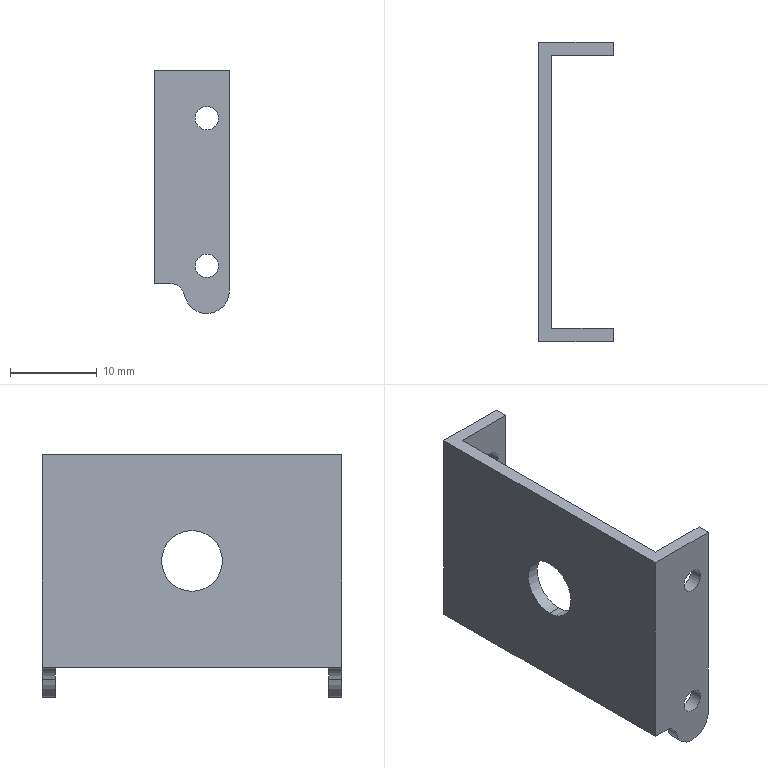Part | SolidWorks | features BaseBody 1 | 1 solid | 24 faces | box 8.6 x 34.5 x 28 mm | volume 1746 mm3 | cylinder 14 | plane 10 | commonest cylinder face diameters 2.7 x8 3.485 x2 5.2 x2 7 x2
STEP:
#1=CARTESIAN_POINT('',(1.5,17.25,-1.757));
#2=VERTEX_POINT('',#1);
#3=CARTESIAN_POINT('',(1.5,17.25,5.243));
#4=VERTEX_POINT('',#3);
#5=CARTESIAN_POINT('',(1.5,17.25,1.743));
#6=DIRECTION('',(-1.,0.,0.));
#7=DIRECTION('',(0.,-1.,0.));
#8=AXIS2_PLACEMENT_3D('',#5,#6,#7);
#9=CIRCLE('',#8,3.5);
#10=EDGE_CURVE('',#2,#4,#9,.T.);
#11=ORIENTED_EDGE('',*,*,#10,.F.);
#12=CARTESIAN_POINT('',(0.,17.25,-1.757));
#13=VERTEX_POINT('',#12);
#14=CARTESIAN_POINT('',(8.6,17.25,-1.757));
#15=DIRECTION('',(-1.,0.,0.));
#16=VECTOR('',#15,1000.);
#17=LINE('',#14,#16);
#18=EDGE_CURVE('',#2,#13,#17,.T.);
#19=ORIENTED_EDGE('',*,*,#18,.T.);
#20=CARTESIAN_POINT('',(0.,17.25,5.243));
#21=VERTEX_POINT('',#20);
#22=CARTESIAN_POINT('',(0.,17.25,1.743));
#23=DIRECTION('',(-1.,0.,0.));
#24=DIRECTION('',(0.,0.,1.));
#25=AXIS2_PLACEMENT_3D('',#22,#23,#24);
#26=CIRCLE('',#25,3.5);
#27=EDGE_CURVE('',#13,#21,#26,.T.);
#28=ORIENTED_EDGE('',*,*,#27,.T.);
#29=CARTESIAN_POINT('',(8.6,17.25,5.243));
#30=DIRECTION('',(-1.,0.,0.));
#31=VECTOR('',#30,1000.);
#32=LINE('',#29,#31);
#33=EDGE_CURVE('',#4,#21,#32,.T.);
#34=ORIENTED_EDGE('',*,*,#33,.F.);
#35=EDGE_LOOP('',(#11,#19,#28,#34));
#36=FACE_OUTER_BOUND('',#35,.T.);
#37=CARTESIAN_POINT('',(8.6,17.25,1.743));
#38=DIRECTION('',(-1.,0.,0.));
#39=DIRECTION('',(0.,0.,1.));
#40=AXIS2_PLACEMENT_3D('',#37,#38,#39);
#41=CYLINDRICAL_SURFACE('',#40,3.5);
#42=ADVANCED_FACE('',(#36),#41,.F.);
#43=CARTESIAN_POINT('',(7.35,0.,8.5));
#44=VERTEX_POINT('',#43);
#45=CARTESIAN_POINT('',(4.65,0.,8.5));
#46=VERTEX_POINT('',#45);
#47=CARTESIAN_POINT('',(6.,0.,8.5));
#48=DIRECTION('',(0.,1.,0.));
#49=DIRECTION('',(-1.,0.,0.));
#50=AXIS2_PLACEMENT_3D('',#47,#48,#49);
#51=CIRCLE('',#50,1.35);
#52=EDGE_CURVE('',#44,#46,#51,.T.);
#53=ORIENTED_EDGE('',*,*,#52,.F.);
#54=CARTESIAN_POINT('',(7.35,1.5,8.5));
#55=VERTEX_POINT('',#54);
#56=CARTESIAN_POINT('',(7.35,0.,8.5));
#57=DIRECTION('',(0.,1.,0.));
#58=VECTOR('',#57,1000.);
#59=LINE('',#56,#58);
#60=EDGE_CURVE('',#44,#55,#59,.T.);
#61=ORIENTED_EDGE('',*,*,#60,.T.);
#62=CARTESIAN_POINT('',(4.65,1.5,8.5));
#63=VERTEX_POINT('',#62);
#64=CARTESIAN_POINT('',(6.,1.5,8.5));
#65=DIRECTION('',(0.,-1.,0.));
#66=DIRECTION('',(0.,0.,-1.));
#67=AXIS2_PLACEMENT_3D('',#64,#65,#66);
#68=CIRCLE('',#67,1.35);
#69=EDGE_CURVE('',#63,#55,#68,.T.);
#70=ORIENTED_EDGE('',*,*,#69,.F.);
#71=CARTESIAN_POINT('',(4.65,0.,8.5));
#72=DIRECTION('',(0.,1.,0.));
#73=VECTOR('',#72,1000.);
#74=LINE('',#71,#73);
#75=EDGE_CURVE('',#46,#63,#74,.T.);
#76=ORIENTED_EDGE('',*,*,#75,.F.);
#77=EDGE_LOOP('',(#53,#61,#70,#76));
#78=FACE_OUTER_BOUND('',#77,.T.);
#79=CARTESIAN_POINT('',(6.,0.,8.5));
#80=DIRECTION('',(0.,1.,0.));
#81=DIRECTION('',(-1.,0.,0.));
#82=AXIS2_PLACEMENT_3D('',#79,#80,#81);
#83=CYLINDRICAL_SURFACE('',#82,1.35);
#84=ADVANCED_FACE('',(#78),#83,.F.);
#85=CARTESIAN_POINT('',(7.35,33.,8.5));
#86=VERTEX_POINT('',#85);
#87=CARTESIAN_POINT('',(4.65,33.,8.5));
#88=VERTEX_POINT('',#87);
#89=CARTESIAN_POINT('',(6.,33.,8.5));
#90=DIRECTION('',(0.,1.,0.));
#91=DIRECTION('',(0.,0.,1.));
#92=AXIS2_PLACEMENT_3D('',#89,#90,#91);
#93=CIRCLE('',#92,1.35);
#94=EDGE_CURVE('',#86,#88,#93,.T.);
#95=ORIENTED_EDGE('',*,*,#94,.F.);
#96=CARTESIAN_POINT('',(7.35,34.5,8.5));
#97=VERTEX_POINT('',#96);
#98=CARTESIAN_POINT('',(7.35,0.,8.5));
#99=DIRECTION('',(0.,1.,0.));
#100=VECTOR('',#99,1000.);
#101=LINE('',#98,#100);
#102=EDGE_CURVE('',#86,#97,#101,.T.);
#103=ORIENTED_EDGE('',*,*,#102,.T.);
#104=CARTESIAN_POINT('',(4.65,34.5,8.5));
#105=VERTEX_POINT('',#104);
#106=CARTESIAN_POINT('',(6.,34.5,8.5));
#107=DIRECTION('',(0.,1.,0.));
#108=DIRECTION('',(-1.,0.,0.));
#109=AXIS2_PLACEMENT_3D('',#106,#107,#108);
#110=CIRCLE('',#109,1.35);
#111=EDGE_CURVE('',#97,#105,#110,.T.);
#112=ORIENTED_EDGE('',*,*,#111,.T.);
#113=CARTESIAN_POINT('',(4.65,0.,8.5));
#114=DIRECTION('',(0.,1.,0.));
#115=VECTOR('',#114,1000.);
#116=LINE('',#113,#115);
#117=EDGE_CURVE('',#88,#105,#116,.T.);
#118=ORIENTED_EDGE('',*,*,#117,.F.);
#119=EDGE_LOOP('',(#95,#103,#112,#118));
#120=FACE_OUTER_BOUND('',#119,.T.);
#121=CARTESIAN_POINT('',(6.,0.,8.5));
#122=DIRECTION('',(0.,1.,0.));
#123=DIRECTION('',(-1.,0.,0.));
#124=AXIS2_PLACEMENT_3D('',#121,#122,#123);
#125=CYLINDRICAL_SURFACE('',#124,1.35);
#126=ADVANCED_FACE('',(#120),#125,.F.);
#127=CARTESIAN_POINT('',(7.35,0.,-8.5));
#128=VERTEX_POINT('',#127);
#129=CARTESIAN_POINT('',(4.65,0.,-8.5));
#130=VERTEX_POINT('',#129);
#131=CARTESIAN_POINT('',(6.,0.,-8.5));
#132=DIRECTION('',(0.,1.,0.));
#133=DIRECTION('',(-1.,0.,0.));
#134=AXIS2_PLACEMENT_3D('',#131,#132,#133);
#135=CIRCLE('',#134,1.35);
#136=EDGE_CURVE('',#128,#130,#135,.T.);
#137=ORIENTED_EDGE('',*,*,#136,.F.);
#138=CARTESIAN_POINT('',(7.35,1.5,-8.5));
#139=VERTEX_POINT('',#138);
#140=CARTESIAN_POINT('',(7.35,0.,-8.5));
#141=DIRECTION('',(0.,1.,0.));
#142=VECTOR('',#141,1000.);
#143=LINE('',#140,#142);
#144=EDGE_CURVE('',#128,#139,#143,.T.);
#145=ORIENTED_EDGE('',*,*,#144,.T.);
#146=CARTESIAN_POINT('',(4.65,1.5,-8.5));
#147=VERTEX_POINT('',#146);
#148=CARTESIAN_POINT('',(6.,1.5,-8.5));
#149=DIRECTION('',(0.,-1.,0.));
#150=DIRECTION('',(0.,0.,-1.));
#151=AXIS2_PLACEMENT_3D('',#148,#149,#150);
#152=CIRCLE('',#151,1.35);
#153=EDGE_CURVE('',#147,#139,#152,.T.);
#154=ORIENTED_EDGE('',*,*,#153,.F.);
#155=CARTESIAN_POINT('',(4.65,0.,-8.5));
#156=DIRECTION('',(0.,1.,0.));
#157=VECTOR('',#156,1000.);
#158=LINE('',#155,#157);
#159=EDGE_CURVE('',#130,#147,#158,.T.);
#160=ORIENTED_EDGE('',*,*,#159,.F.);
#161=EDGE_LOOP('',(#137,#145,#154,#160));
#162=FACE_OUTER_BOUND('',#161,.T.);
#163=CARTESIAN_POINT('',(6.,0.,-8.5));
#164=DIRECTION('',(0.,1.,0.));
#165=DIRECTION('',(-1.,0.,0.));
#166=AXIS2_PLACEMENT_3D('',#163,#164,#165);
#167=CYLINDRICAL_SURFACE('',#166,1.35);
#168=ADVANCED_FACE('',(#162),#167,.F.);
#169=CARTESIAN_POINT('',(7.35,33.,-8.5));
#170=VERTEX_POINT('',#169);
#171=CARTESIAN_POINT('',(4.65,33.,-8.5));
#172=VERTEX_POINT('',#171);
#173=CARTESIAN_POINT('',(6.,33.,-8.5));
#174=DIRECTION('',(0.,1.,0.));
#175=DIRECTION('',(0.,0.,1.));
#176=AXIS2_PLACEMENT_3D('',#173,#174,#175);
#177=CIRCLE('',#176,1.35);
#178=EDGE_CURVE('',#170,#172,#177,.T.);
#179=ORIENTED_EDGE('',*,*,#178,.F.);
#180=CARTESIAN_POINT('',(7.35,34.5,-8.5));
#181=VERTEX_POINT('',#180);
#182=CARTESIAN_POINT('',(7.35,0.,-8.5));
#183=DIRECTION('',(0.,1.,0.));
#184=VECTOR('',#183,1000.);
#185=LINE('',#182,#184);
#186=EDGE_CURVE('',#170,#181,#185,.T.);
#187=ORIENTED_EDGE('',*,*,#186,.T.);
#188=CARTESIAN_POINT('',(4.65,34.5,-8.5));
#189=VERTEX_POINT('',#188);
#190=CARTESIAN_POINT('',(6.,34.5,-8.5));
#191=DIRECTION('',(0.,1.,0.));
#192=DIRECTION('',(-1.,0.,0.));
#193=AXIS2_PLACEMENT_3D('',#190,#191,#192);
#194=CIRCLE('',#193,1.35);
#195=EDGE_CURVE('',#181,#189,#194,.T.);
#196=ORIENTED_EDGE('',*,*,#195,.T.);
#197=CARTESIAN_POINT('',(4.65,0.,-8.5));
#198=DIRECTION('',(0.,1.,0.));
#199=VECTOR('',#198,1000.);
#200=LINE('',#197,#199);
#201=EDGE_CURVE('',#172,#189,#200,.T.);
#202=ORIENTED_EDGE('',*,*,#201,.F.);
#203=EDGE_LOOP('',(#179,#187,#196,#202));
#204=FACE_OUTER_BOUND('',#203,.T.);
#205=CARTESIAN_POINT('',(6.,0.,-8.5));
#206=DIRECTION('',(0.,1.,0.));
#207=DIRECTION('',(-1.,0.,0.));
#208=AXIS2_PLACEMENT_3D('',#205,#206,#207);
#209=CYLINDRICAL_SURFACE('',#208,1.35);
#210=ADVANCED_FACE('',(#204),#209,.F.);
#211=CARTESIAN_POINT('',(6.,0.,8.5));
#212=DIRECTION('',(0.,1.,0.));
#213=DIRECTION('',(-1.,0.,0.));
#214=AXIS2_PLACEMENT_3D('',#211,#212,#213);
#215=CIRCLE('',#214,1.35);
#216=EDGE_CURVE('',#46,#44,#215,.T.);
#217=ORIENTED_EDGE('',*,*,#216,.T.);
#218=ORIENTED_EDGE('',*,*,#52,.T.);
#219=EDGE_LOOP('',(#217,#218));
#220=FACE_BOUND('',#219,.T.);
#221=CARTESIAN_POINT('',(6.,0.,-8.5));
#222=DIRECTION('',(0.,1.,0.));
#223=DIRECTION('',(-1.,0.,0.));
#224=AXIS2_PLACEMENT_3D('',#221,#222,#223);
#225=CIRCLE('',#224,1.35);
#226=EDGE_CURVE('',#130,#128,#225,.T.);
#227=ORIENTED_EDGE('',*,*,#226,.T.);
#228=ORIENTED_EDGE('',*,*,#136,.T.);
#229=EDGE_LOOP('',(#227,#228));
#230=FACE_BOUND('',#229,.T.);
#231=CARTESIAN_POINT('',(8.6,0.,-11.4));
#232=VERTEX_POINT('',#231);
#233=CARTESIAN_POINT('',(3.451,0.,-11.913));
#234=VERTEX_POINT('',#233);
#235=CARTESIAN_POINT('',(6.,0.,-11.4));
#236=DIRECTION('',(0.,1.,0.));
#237=DIRECTION('',(0.,0.,1.));
#238=AXIS2_PLACEMENT_3D('',#235,#236,#237);
#239=CIRCLE('',#238,2.6);
#240=EDGE_CURVE('',#232,#234,#239,.T.);
#241=ORIENTED_EDGE('',*,*,#240,.F.);
#242=CARTESIAN_POINT('',(8.6,0.,14.));
#243=VERTEX_POINT('',#242);
#244=CARTESIAN_POINT('',(8.6,0.,14.));
#245=DIRECTION('',(0.,0.,-1.));
#246=VECTOR('',#245,1000.);
#247=LINE('',#244,#246);
#248=EDGE_CURVE('',#243,#232,#247,.T.);
#249=ORIENTED_EDGE('',*,*,#248,.F.);
#250=CARTESIAN_POINT('',(0.,0.,14.));
#251=VERTEX_POINT('',#250);
#252=CARTESIAN_POINT('',(8.6,0.,14.));
#253=DIRECTION('',(1.,0.,0.));
#254=VECTOR('',#253,1000.);
#255=LINE('',#252,#254);
#256=EDGE_CURVE('',#251,#243,#255,.T.);
#257=ORIENTED_EDGE('',*,*,#256,.F.);
#258=CARTESIAN_POINT('',(0.,0.,-10.515));
#259=VERTEX_POINT('',#258);
#260=CARTESIAN_POINT('',(0.,0.,14.));
#261=DIRECTION('',(0.,0.,-1.));
#262=VECTOR('',#261,1000.);
#263=LINE('',#260,#262);
#264=EDGE_CURVE('',#251,#259,#263,.T.);
#265=ORIENTED_EDGE('',*,*,#264,.T.);
#266=CARTESIAN_POINT('',(1.743,0.,-10.515));
#267=VERTEX_POINT('',#266);
#268=CARTESIAN_POINT('',(0.,0.,-10.515));
#269=DIRECTION('',(-1.,0.,0.));
#270=VECTOR('',#269,1000.);
#271=LINE('',#268,#270);
#272=EDGE_CURVE('',#267,#259,#271,.T.);
#273=ORIENTED_EDGE('',*,*,#272,.F.);
#274=CARTESIAN_POINT('',(1.743,0.,-12.257));
#275=DIRECTION('',(0.,1.,0.));
#276=DIRECTION('',(0.,0.,1.));
#277=AXIS2_PLACEMENT_3D('',#274,#275,#276);
#278=CIRCLE('',#277,1.743);
#279=EDGE_CURVE('',#267,#234,#278,.T.);
#280=ORIENTED_EDGE('',*,*,#279,.T.);
#281=EDGE_LOOP('',(#241,#249,#257,#265,#273,#280));
#282=FACE_OUTER_BOUND('',#281,.T.);
#283=CARTESIAN_POINT('',(8.6,0.,14.));
#284=DIRECTION('',(0.,1.,0.));
#285=DIRECTION('',(-1.,0.,0.));
#286=AXIS2_PLACEMENT_3D('',#283,#284,#285);
#287=PLANE('',#286);
#288=ADVANCED_FACE('',(#220,#230,#282),#287,.F.);
#289=ORIENTED_EDGE('',*,*,#69,.T.);
#290=CARTESIAN_POINT('',(6.,1.5,8.5));
#291=DIRECTION('',(0.,-1.,0.));
#292=DIRECTION('',(0.,0.,-1.));
#293=AXIS2_PLACEMENT_3D('',#290,#291,#292);
#294=CIRCLE('',#293,1.35);
#295=EDGE_CURVE('',#55,#63,#294,.T.);
#296=ORIENTED_EDGE('',*,*,#295,.T.);
#297=EDGE_LOOP('',(#289,#296));
#298=FACE_BOUND('',#297,.T.);
#299=ORIENTED_EDGE('',*,*,#153,.T.);
#300=CARTESIAN_POINT('',(6.,1.5,-8.5));
#301=DIRECTION('',(0.,-1.,0.));
#302=DIRECTION('',(0.,0.,-1.));
#303=AXIS2_PLACEMENT_3D('',#300,#301,#302);
#304=CIRCLE('',#303,1.35);
#305=EDGE_CURVE('',#139,#147,#304,.T.);
#306=ORIENTED_EDGE('',*,*,#305,.T.);
#307=EDGE_LOOP('',(#299,#306));
#308=FACE_BOUND('',#307,.T.);
#309=CARTESIAN_POINT('',(8.6,1.5,14.));
#310=VERTEX_POINT('',#309);
#311=CARTESIAN_POINT('',(8.6,1.5,-11.4));
#312=VERTEX_POINT('',#311);
#313=CARTESIAN_POINT('',(8.6,1.5,14.));
#314=DIRECTION('',(0.,0.,-1.));
#315=VECTOR('',#314,1000.);
#316=LINE('',#313,#315);
#317=EDGE_CURVE('',#310,#312,#316,.T.);
#318=ORIENTED_EDGE('',*,*,#317,.T.);
#319=CARTESIAN_POINT('',(3.451,1.5,-11.913));
#320=VERTEX_POINT('',#319);
#321=CARTESIAN_POINT('',(6.,1.5,-11.4));
#322=DIRECTION('',(0.,-1.,0.));
#323=DIRECTION('',(0.,0.,-1.));
#324=AXIS2_PLACEMENT_3D('',#321,#322,#323);
#325=CIRCLE('',#324,2.6);
#326=EDGE_CURVE('',#320,#312,#325,.T.);
#327=ORIENTED_EDGE('',*,*,#326,.F.);
#328=CARTESIAN_POINT('',(1.743,1.5,-10.515));
#329=VERTEX_POINT('',#328);
#330=CARTESIAN_POINT('',(1.743,1.5,-12.257));
#331=DIRECTION('',(0.,-1.,0.));
#332=DIRECTION('',(0.,0.,-1.));
#333=AXIS2_PLACEMENT_3D('',#330,#331,#332);
#334=CIRCLE('',#333,1.743);
#335=EDGE_CURVE('',#320,#329,#334,.T.);
#336=ORIENTED_EDGE('',*,*,#335,.T.);
#337=CARTESIAN_POINT('',(1.5,1.5,-10.515));
#338=VERTEX_POINT('',#337);
#339=CARTESIAN_POINT('',(1.5,1.5,-10.515));
#340=DIRECTION('',(1.,0.,0.));
#341=VECTOR('',#340,1000.);
#342=LINE('',#339,#341);
#343=EDGE_CURVE('',#338,#329,#342,.T.);
#344=ORIENTED_EDGE('',*,*,#343,.F.);
#345=CARTESIAN_POINT('',(1.5,1.5,14.));
#346=VERTEX_POINT('',#345);
#347=CARTESIAN_POINT('',(1.5,1.5,14.));
#348=DIRECTION('',(0.,0.,-1.));
#349=VECTOR('',#348,1000.);
#350=LINE('',#347,#349);
#351=EDGE_CURVE('',#346,#338,#350,.T.);
#352=ORIENTED_EDGE('',*,*,#351,.F.);
#353=CARTESIAN_POINT('',(1.5,1.5,14.));
#354=DIRECTION('',(-1.,0.,0.));
#355=VECTOR('',#354,1000.);
#356=LINE('',#353,#355);
#357=EDGE_CURVE('',#310,#346,#356,.T.);
#358=ORIENTED_EDGE('',*,*,#357,.F.);
#359=EDGE_LOOP('',(#318,#327,#336,#344,#352,#358));
#360=FACE_OUTER_BOUND('',#359,.T.);
#361=CARTESIAN_POINT('',(1.5,1.5,14.));
#362=DIRECTION('',(0.,-1.,0.));
#363=DIRECTION('',(0.,0.,-1.));
#364=AXIS2_PLACEMENT_3D('',#361,#362,#363);
#365=PLANE('',#364);
#366=ADVANCED_FACE('',(#298,#308,#360),#365,.F.);
#367=CARTESIAN_POINT('',(1.5,17.25,1.743));
#368=DIRECTION('',(-1.,0.,0.));
#369=DIRECTION('',(0.,-1.,0.));
#370=AXIS2_PLACEMENT_3D('',#367,#368,#369);
#371=CIRCLE('',#370,3.5);
#372=EDGE_CURVE('',#4,#2,#371,.T.);
#373=ORIENTED_EDGE('',*,*,#372,.T.);
#374=ORIENTED_EDGE('',*,*,#10,.T.);
#375=EDGE_LOOP('',(#373,#374));
#376=FACE_BOUND('',#375,.T.);
#377=CARTESIAN_POINT('',(1.5,33.,-10.515));
#378=VERTEX_POINT('',#377);
#379=CARTESIAN_POINT('',(1.5,33.,-10.515));
#380=DIRECTION('',(0.,-1.,0.));
#381=VECTOR('',#380,1000.);
#382=LINE('',#379,#381);
#383=EDGE_CURVE('',#378,#338,#382,.T.);
#384=ORIENTED_EDGE('',*,*,#383,.F.);
#385=CARTESIAN_POINT('',(1.5,33.,14.));
#386=VERTEX_POINT('',#385);
#387=CARTESIAN_POINT('',(1.5,33.,14.));
#388=DIRECTION('',(0.,0.,-1.));
#389=VECTOR('',#388,1000.);
#390=LINE('',#387,#389);
#391=EDGE_CURVE('',#386,#378,#390,.T.);
#392=ORIENTED_EDGE('',*,*,#391,.F.);
#393=CARTESIAN_POINT('',(1.5,33.,14.));
#394=DIRECTION('',(0.,1.,0.));
#395=VECTOR('',#394,1000.);
#396=LINE('',#393,#395);
#397=EDGE_CURVE('',#346,#386,#396,.T.);
#398=ORIENTED_EDGE('',*,*,#397,.F.);
#399=ORIENTED_EDGE('',*,*,#351,.T.);
#400=EDGE_LOOP('',(#384,#392,#398,#399));
#401=FACE_OUTER_BOUND('',#400,.T.);
#402=CARTESIAN_POINT('',(1.5,33.,14.));
#403=DIRECTION('',(-1.,0.,0.));
#404=DIRECTION('',(0.,-1.,0.));
#405=AXIS2_PLACEMENT_3D('',#402,#403,#404);
#406=PLANE('',#405);
#407=ADVANCED_FACE('',(#376,#401),#406,.F.);
#408=CARTESIAN_POINT('',(6.,33.,8.5));
#409=DIRECTION('',(0.,1.,0.));
#410=DIRECTION('',(0.,0.,1.));
#411=AXIS2_PLACEMENT_3D('',#408,#409,#410);
#412=CIRCLE('',#411,1.35);
#413=EDGE_CURVE('',#88,#86,#412,.T.);
#414=ORIENTED_EDGE('',*,*,#413,.T.);
#415=ORIENTED_EDGE('',*,*,#94,.T.);
#416=EDGE_LOOP('',(#414,#415));
#417=FACE_BOUND('',#416,.T.);
#418=CARTESIAN_POINT('',(6.,33.,-8.5));
#419=DIRECTION('',(0.,1.,0.));
#420=DIRECTION('',(0.,0.,1.));
#421=AXIS2_PLACEMENT_3D('',#418,#419,#420);
#422=CIRCLE('',#421,1.35);
#423=EDGE_CURVE('',#172,#170,#422,.T.);
#424=ORIENTED_EDGE('',*,*,#423,.T.);
#425=ORIENTED_EDGE('',*,*,#178,.T.);
#426=EDGE_LOOP('',(#424,#425));
#427=FACE_BOUND('',#426,.T.);
#428=CARTESIAN_POINT('',(8.6,33.,-11.4));
#429=VERTEX_POINT('',#428);
#430=CARTESIAN_POINT('',(3.451,33.,-11.913));
#431=VERTEX_POINT('',#430);
#432=CARTESIAN_POINT('',(6.,33.,-11.4));
#433=DIRECTION('',(0.,1.,0.));
#434=DIRECTION('',(0.,0.,1.));
#435=AXIS2_PLACEMENT_3D('',#432,#433,#434);
#436=CIRCLE('',#435,2.6);
#437=EDGE_CURVE('',#429,#431,#436,.T.);
#438=ORIENTED_EDGE('',*,*,#437,.F.);
#439=CARTESIAN_POINT('',(8.6,33.,14.));
#440=VERTEX_POINT('',#439);
#441=CARTESIAN_POINT('',(8.6,33.,14.));
#442=DIRECTION('',(0.,0.,-1.));
#443=VECTOR('',#442,1000.);
#444=LINE('',#441,#443);
#445=EDGE_CURVE('',#440,#429,#444,.T.);
#446=ORIENTED_EDGE('',*,*,#445,.F.);
#447=CARTESIAN_POINT('',(8.6,33.,14.));
#448=DIRECTION('',(1.,0.,0.));
#449=VECTOR('',#448,1000.);
#450=LINE('',#447,#449);
#451=EDGE_CURVE('',#386,#440,#450,.T.);
#452=ORIENTED_EDGE('',*,*,#451,.F.);
#453=ORIENTED_EDGE('',*,*,#391,.T.);
#454=CARTESIAN_POINT('',(1.743,33.,-10.515));
#455=VERTEX_POINT('',#454);
#456=CARTESIAN_POINT('',(8.6,33.,-10.515));
#457=DIRECTION('',(-1.,0.,0.));
#458=VECTOR('',#457,1000.);
#459=LINE('',#456,#458);
#460=EDGE_CURVE('',#455,#378,#459,.T.);
#461=ORIENTED_EDGE('',*,*,#460,.F.);
#462=CARTESIAN_POINT('',(1.743,33.,-12.257));
#463=DIRECTION('',(0.,1.,0.));
#464=DIRECTION('',(0.,0.,1.));
#465=AXIS2_PLACEMENT_3D('',#462,#463,#464);
#466=CIRCLE('',#465,1.743);
#467=EDGE_CURVE('',#455,#431,#466,.T.);
#468=ORIENTED_EDGE('',*,*,#467,.T.);
#469=EDGE_LOOP('',(#438,#446,#452,#453,#461,#468));
#470=FACE_OUTER_BOUND('',#469,.T.);
#471=CARTESIAN_POINT('',(8.6,33.,14.));
#472=DIRECTION('',(0.,1.,0.));
#473=DIRECTION('',(0.,0.,1.));
#474=AXIS2_PLACEMENT_3D('',#471,#472,#473);
#475=PLANE('',#474);
#476=ADVANCED_FACE('',(#417,#427,#470),#475,.F.);
#477=CARTESIAN_POINT('',(6.,34.5,8.5));
#478=DIRECTION('',(0.,1.,0.));
#479=DIRECTION('',(-1.,0.,0.));
#480=AXIS2_PLACEMENT_3D('',#477,#478,#479);
#481=CIRCLE('',#480,1.35);
#482=EDGE_CURVE('',#105,#97,#481,.T.);
#483=ORIENTED_EDGE('',*,*,#482,.F.);
#484=ORIENTED_EDGE('',*,*,#111,.F.);
#485=EDGE_LOOP('',(#483,#484));
#486=FACE_BOUND('',#485,.T.);
#487=CARTESIAN_POINT('',(6.,34.5,-8.5));
#488=DIRECTION('',(0.,1.,0.));
#489=DIRECTION('',(-1.,0.,0.));
#490=AXIS2_PLACEMENT_3D('',#487,#488,#489);
#491=CIRCLE('',#490,1.35);
#492=EDGE_CURVE('',#189,#181,#491,.T.);
#493=ORIENTED_EDGE('',*,*,#492,.F.);
#494=ORIENTED_EDGE('',*,*,#195,.F.);
#495=EDGE_LOOP('',(#493,#494));
#496=FACE_BOUND('',#495,.T.);
#497=CARTESIAN_POINT('',(8.6,34.5,-11.4));
#498=VERTEX_POINT('',#497);
#499=CARTESIAN_POINT('',(3.451,34.5,-11.913));
#500=VERTEX_POINT('',#499);
#501=CARTESIAN_POINT('',(6.,34.5,-11.4));
#502=DIRECTION('',(0.,1.,0.));
#503=DIRECTION('',(0.,0.,1.));
#504=AXIS2_PLACEMENT_3D('',#501,#502,#503);
#505=CIRCLE('',#504,2.6);
#506=EDGE_CURVE('',#498,#500,#505,.T.);
#507=ORIENTED_EDGE('',*,*,#506,.T.);
#508=CARTESIAN_POINT('',(1.743,34.5,-10.515));
#509=VERTEX_POINT('',#508);
#510=CARTESIAN_POINT('',(1.743,34.5,-12.257));
#511=DIRECTION('',(0.,1.,0.));
#512=DIRECTION('',(0.,0.,1.));
#513=AXIS2_PLACEMENT_3D('',#510,#511,#512);
#514=CIRCLE('',#513,1.743);
#515=EDGE_CURVE('',#509,#500,#514,.T.);
#516=ORIENTED_EDGE('',*,*,#515,.F.);
#517=CARTESIAN_POINT('',(0.,34.5,-10.515));
#518=VERTEX_POINT('',#517);
#519=CARTESIAN_POINT('',(0.,34.5,-10.515));
#520=DIRECTION('',(-1.,0.,0.));
#521=VECTOR('',#520,1000.);
#522=LINE('',#519,#521);
#523=EDGE_CURVE('',#509,#518,#522,.T.);
#524=ORIENTED_EDGE('',*,*,#523,.T.);
#525=CARTESIAN_POINT('',(0.,34.5,14.));
#526=VERTEX_POINT('',#525);
#527=CARTESIAN_POINT('',(0.,34.5,14.));
#528=DIRECTION('',(0.,0.,-1.));
#529=VECTOR('',#528,1000.);
#530=LINE('',#527,#529);
#531=EDGE_CURVE('',#526,#518,#530,.T.);
#532=ORIENTED_EDGE('',*,*,#531,.F.);
#533=CARTESIAN_POINT('',(8.6,34.5,14.));
#534=VERTEX_POINT('',#533);
#535=CARTESIAN_POINT('',(0.,34.5,14.));
#536=DIRECTION('',(-1.,0.,0.));
#537=VECTOR('',#536,1000.);
#538=LINE('',#535,#537);
#539=EDGE_CURVE('',#534,#526,#538,.T.);
#540=ORIENTED_EDGE('',*,*,#539,.F.);
#541=CARTESIAN_POINT('',(8.6,34.5,14.));
#542=DIRECTION('',(0.,0.,-1.));
#543=VECTOR('',#542,1000.);
#544=LINE('',#541,#543);
#545=EDGE_CURVE('',#534,#498,#544,.T.);
#546=ORIENTED_EDGE('',*,*,#545,.T.);
#547=EDGE_LOOP('',(#507,#516,#524,#532,#540,#546));
#548=FACE_OUTER_BOUND('',#547,.T.);
#549=CARTESIAN_POINT('',(0.,34.5,14.));
#550=DIRECTION('',(0.,-1.,0.));
#551=DIRECTION('',(0.,0.,-1.));
#552=AXIS2_PLACEMENT_3D('',#549,#550,#551);
#553=PLANE('',#552);
#554=ADVANCED_FACE('',(#486,#496,#548),#553,.F.);
#555=CARTESIAN_POINT('',(0.,17.25,1.743));
#556=DIRECTION('',(-1.,0.,0.));
#557=DIRECTION('',(0.,0.,1.));
#558=AXIS2_PLACEMENT_3D('',#555,#556,#557);
#559=CIRCLE('',#558,3.5);
#560=EDGE_CURVE('',#21,#13,#559,.T.);
#561=ORIENTED_EDGE('',*,*,#560,.F.);
#562=ORIENTED_EDGE('',*,*,#27,.F.);
#563=EDGE_LOOP('',(#561,#562));
#564=FACE_BOUND('',#563,.T.);
#565=CARTESIAN_POINT('',(0.,0.,-10.515));
#566=DIRECTION('',(0.,1.,0.));
#567=VECTOR('',#566,1000.);
#568=LINE('',#565,#567);
#569=EDGE_CURVE('',#259,#518,#568,.T.);
#570=ORIENTED_EDGE('',*,*,#569,.F.);
#571=ORIENTED_EDGE('',*,*,#264,.F.);
#572=CARTESIAN_POINT('',(0.,0.,14.));
#573=DIRECTION('',(0.,-1.,0.));
#574=VECTOR('',#573,1000.);
#575=LINE('',#572,#574);
#576=EDGE_CURVE('',#526,#251,#575,.T.);
#577=ORIENTED_EDGE('',*,*,#576,.F.);
#578=ORIENTED_EDGE('',*,*,#531,.T.);
#579=EDGE_LOOP('',(#570,#571,#577,#578));
#580=FACE_OUTER_BOUND('',#579,.T.);
#581=CARTESIAN_POINT('',(0.,0.,14.));
#582=DIRECTION('',(1.,0.,0.));
#583=DIRECTION('',(0.,0.,-1.));
#584=AXIS2_PLACEMENT_3D('',#581,#582,#583);
#585=PLANE('',#584);
#586=ADVANCED_FACE('',(#564,#580),#585,.F.);
#587=ORIENTED_EDGE('',*,*,#248,.T.);
#588=CARTESIAN_POINT('',(8.6,0.,-11.4));
#589=DIRECTION('',(0.,1.,0.));
#590=VECTOR('',#589,1000.);
#591=LINE('',#588,#590);
#592=EDGE_CURVE('',#232,#312,#591,.T.);
#593=ORIENTED_EDGE('',*,*,#592,.T.);
#594=ORIENTED_EDGE('',*,*,#317,.F.);
#595=CARTESIAN_POINT('',(8.6,1.5,14.));
#596=DIRECTION('',(0.,1.,0.));
#597=VECTOR('',#596,1000.);
#598=LINE('',#595,#597);
#599=EDGE_CURVE('',#243,#310,#598,.T.);
#600=ORIENTED_EDGE('',*,*,#599,.F.);
#601=EDGE_LOOP('',(#587,#593,#594,#600));
#602=FACE_OUTER_BOUND('',#601,.T.);
#603=CARTESIAN_POINT('',(8.6,1.5,14.));
#604=DIRECTION('',(-1.,0.,0.));
#605=DIRECTION('',(0.,0.,1.));
#606=AXIS2_PLACEMENT_3D('',#603,#604,#605);
#607=PLANE('',#606);
#608=ADVANCED_FACE('',(#602),#607,.F.);
#609=ORIENTED_EDGE('',*,*,#445,.T.);
#610=CARTESIAN_POINT('',(8.6,0.,-11.4));
#611=DIRECTION('',(0.,1.,0.));
#612=VECTOR('',#611,1000.);
#613=LINE('',#610,#612);
#614=EDGE_CURVE('',#429,#498,#613,.T.);
#615=ORIENTED_EDGE('',*,*,#614,.T.);
#616=ORIENTED_EDGE('',*,*,#545,.F.);
#617=CARTESIAN_POINT('',(8.6,34.5,14.));
#618=DIRECTION('',(0.,1.,0.));
#619=VECTOR('',#618,1000.);
#620=LINE('',#617,#619);
#621=EDGE_CURVE('',#440,#534,#620,.T.);
#622=ORIENTED_EDGE('',*,*,#621,.F.);
#623=EDGE_LOOP('',(#609,#615,#616,#622));
#624=FACE_OUTER_BOUND('',#623,.T.);
#625=CARTESIAN_POINT('',(8.6,34.5,14.));
#626=DIRECTION('',(-1.,0.,0.));
#627=DIRECTION('',(0.,-1.,0.));
#628=AXIS2_PLACEMENT_3D('',#625,#626,#627);
#629=PLANE('',#628);
#630=ADVANCED_FACE('',(#624),#629,.F.);
#631=ORIENTED_EDGE('',*,*,#256,.T.);
#632=ORIENTED_EDGE('',*,*,#599,.T.);
#633=ORIENTED_EDGE('',*,*,#357,.T.);
#634=ORIENTED_EDGE('',*,*,#397,.T.);
#635=ORIENTED_EDGE('',*,*,#451,.T.);
#636=ORIENTED_EDGE('',*,*,#621,.T.);
#637=ORIENTED_EDGE('',*,*,#539,.T.);
#638=ORIENTED_EDGE('',*,*,#576,.T.);
#639=EDGE_LOOP('',(#631,#632,#633,#634,#635,#636,#637,#638));
#640=FACE_OUTER_BOUND('',#639,.T.);
#641=CARTESIAN_POINT('',(0.,0.,14.));
#642=DIRECTION('',(0.,0.,-1.));
#643=DIRECTION('',(-1.,0.,0.));
#644=AXIS2_PLACEMENT_3D('',#641,#642,#643);
#645=PLANE('',#644);
#646=ADVANCED_FACE('',(#640),#645,.F.);
#647=ORIENTED_EDGE('',*,*,#186,.F.);
#648=ORIENTED_EDGE('',*,*,#423,.F.);
#649=ORIENTED_EDGE('',*,*,#201,.T.);
#650=ORIENTED_EDGE('',*,*,#492,.T.);
#651=EDGE_LOOP('',(#647,#648,#649,#650));
#652=FACE_OUTER_BOUND('',#651,.T.);
#653=CARTESIAN_POINT('',(6.,0.,-8.5));
#654=DIRECTION('',(0.,1.,0.));
#655=DIRECTION('',(-1.,0.,0.));
#656=AXIS2_PLACEMENT_3D('',#653,#654,#655);
#657=CYLINDRICAL_SURFACE('',#656,1.35);
#658=ADVANCED_FACE('',(#652),#657,.F.);
#659=ORIENTED_EDGE('',*,*,#144,.F.);
#660=ORIENTED_EDGE('',*,*,#226,.F.);
#661=ORIENTED_EDGE('',*,*,#159,.T.);
#662=ORIENTED_EDGE('',*,*,#305,.F.);
#663=EDGE_LOOP('',(#659,#660,#661,#662));
#664=FACE_OUTER_BOUND('',#663,.T.);
#665=CARTESIAN_POINT('',(6.,0.,-8.5));
#666=DIRECTION('',(0.,1.,0.));
#667=DIRECTION('',(-1.,0.,0.));
#668=AXIS2_PLACEMENT_3D('',#665,#666,#667);
#669=CYLINDRICAL_SURFACE('',#668,1.35);
#670=ADVANCED_FACE('',(#664),#669,.F.);
#671=ORIENTED_EDGE('',*,*,#102,.F.);
#672=ORIENTED_EDGE('',*,*,#413,.F.);
#673=ORIENTED_EDGE('',*,*,#117,.T.);
#674=ORIENTED_EDGE('',*,*,#482,.T.);
#675=EDGE_LOOP('',(#671,#672,#673,#674));
#676=FACE_OUTER_BOUND('',#675,.T.);
#677=CARTESIAN_POINT('',(6.,0.,8.5));
#678=DIRECTION('',(0.,1.,0.));
#679=DIRECTION('',(-1.,0.,0.));
#680=AXIS2_PLACEMENT_3D('',#677,#678,#679);
#681=CYLINDRICAL_SURFACE('',#680,1.35);
#682=ADVANCED_FACE('',(#676),#681,.F.);
#683=ORIENTED_EDGE('',*,*,#60,.F.);
#684=ORIENTED_EDGE('',*,*,#216,.F.);
#685=ORIENTED_EDGE('',*,*,#75,.T.);
#686=ORIENTED_EDGE('',*,*,#295,.F.);
#687=EDGE_LOOP('',(#683,#684,#685,#686));
#688=FACE_OUTER_BOUND('',#687,.T.);
#689=CARTESIAN_POINT('',(6.,0.,8.5));
#690=DIRECTION('',(0.,1.,0.));
#691=DIRECTION('',(-1.,0.,0.));
#692=AXIS2_PLACEMENT_3D('',#689,#690,#691);
#693=CYLINDRICAL_SURFACE('',#692,1.35);
#694=ADVANCED_FACE('',(#688),#693,.F.);
#695=CARTESIAN_POINT('',(3.451,0.,-11.913));
#696=DIRECTION('',(0.,1.,0.));
#697=VECTOR('',#696,1000.);
#698=LINE('',#695,#697);
#699=EDGE_CURVE('',#234,#320,#698,.T.);
#700=ORIENTED_EDGE('',*,*,#699,.F.);
#701=ORIENTED_EDGE('',*,*,#279,.F.);
#702=CARTESIAN_POINT('',(1.743,0.,-10.515));
#703=DIRECTION('',(0.,1.,0.));
#704=VECTOR('',#703,1000.);
#705=LINE('',#702,#704);
#706=EDGE_CURVE('',#267,#329,#705,.T.);
#707=ORIENTED_EDGE('',*,*,#706,.T.);
#708=ORIENTED_EDGE('',*,*,#335,.F.);
#709=EDGE_LOOP('',(#700,#701,#707,#708));
#710=FACE_OUTER_BOUND('',#709,.T.);
#711=CARTESIAN_POINT('',(1.743,0.,-12.257));
#712=DIRECTION('',(0.,1.,0.));
#713=DIRECTION('',(0.,0.,1.));
#714=AXIS2_PLACEMENT_3D('',#711,#712,#713);
#715=CYLINDRICAL_SURFACE('',#714,1.743);
#716=ADVANCED_FACE('',(#710),#715,.F.);
#717=CARTESIAN_POINT('',(1.743,0.,-10.515));
#718=DIRECTION('',(0.,1.,0.));
#719=VECTOR('',#718,1000.);
#720=LINE('',#717,#719);
#721=EDGE_CURVE('',#455,#509,#720,.T.);
#722=ORIENTED_EDGE('',*,*,#721,.T.);
#723=ORIENTED_EDGE('',*,*,#515,.T.);
#724=CARTESIAN_POINT('',(3.451,0.,-11.913));
#725=DIRECTION('',(0.,1.,0.));
#726=VECTOR('',#725,1000.);
#727=LINE('',#724,#726);
#728=EDGE_CURVE('',#431,#500,#727,.T.);
#729=ORIENTED_EDGE('',*,*,#728,.F.);
#730=ORIENTED_EDGE('',*,*,#467,.F.);
#731=EDGE_LOOP('',(#722,#723,#729,#730));
#732=FACE_OUTER_BOUND('',#731,.T.);
#733=CARTESIAN_POINT('',(1.743,0.,-12.257));
#734=DIRECTION('',(0.,1.,0.));
#735=DIRECTION('',(0.,0.,1.));
#736=AXIS2_PLACEMENT_3D('',#733,#734,#735);
#737=CYLINDRICAL_SURFACE('',#736,1.743);
#738=ADVANCED_FACE('',(#732),#737,.F.);
#739=ORIENTED_EDGE('',*,*,#343,.T.);
#740=ORIENTED_EDGE('',*,*,#706,.F.);
#741=ORIENTED_EDGE('',*,*,#272,.T.);
#742=ORIENTED_EDGE('',*,*,#569,.T.);
#743=ORIENTED_EDGE('',*,*,#523,.F.);
#744=ORIENTED_EDGE('',*,*,#721,.F.);
#745=ORIENTED_EDGE('',*,*,#460,.T.);
#746=ORIENTED_EDGE('',*,*,#383,.T.);
#747=EDGE_LOOP('',(#739,#740,#741,#742,#743,#744,#745,#746));
#748=FACE_OUTER_BOUND('',#747,.T.);
#749=CARTESIAN_POINT('',(0.,0.,-10.515));
#750=DIRECTION('',(0.,0.,-1.));
#751=DIRECTION('',(-1.,0.,0.));
#752=AXIS2_PLACEMENT_3D('',#749,#750,#751);
#753=PLANE('',#752);
#754=ADVANCED_FACE('',(#748),#753,.T.);
#755=ORIENTED_EDGE('',*,*,#326,.T.);
#756=ORIENTED_EDGE('',*,*,#592,.F.);
#757=ORIENTED_EDGE('',*,*,#240,.T.);
#758=ORIENTED_EDGE('',*,*,#699,.T.);
#759=EDGE_LOOP('',(#755,#756,#757,#758));
#760=FACE_OUTER_BOUND('',#759,.T.);
#761=CARTESIAN_POINT('',(6.,0.,-11.4));
#762=DIRECTION('',(0.,1.,0.));
#763=DIRECTION('',(0.,0.,1.));
#764=AXIS2_PLACEMENT_3D('',#761,#762,#763);
#765=CYLINDRICAL_SURFACE('',#764,2.6);
#766=ADVANCED_FACE('',(#760),#765,.T.);
#767=ORIENTED_EDGE('',*,*,#437,.T.);
#768=ORIENTED_EDGE('',*,*,#728,.T.);
#769=ORIENTED_EDGE('',*,*,#506,.F.);
#770=ORIENTED_EDGE('',*,*,#614,.F.);
#771=EDGE_LOOP('',(#767,#768,#769,#770));
#772=FACE_OUTER_BOUND('',#771,.T.);
#773=CARTESIAN_POINT('',(6.,0.,-11.4));
#774=DIRECTION('',(0.,1.,0.));
#775=DIRECTION('',(0.,0.,1.));
#776=AXIS2_PLACEMENT_3D('',#773,#774,#775);
#777=CYLINDRICAL_SURFACE('',#776,2.6);
#778=ADVANCED_FACE('',(#772),#777,.T.);
#779=ORIENTED_EDGE('',*,*,#18,.F.);
#780=ORIENTED_EDGE('',*,*,#372,.F.);
#781=ORIENTED_EDGE('',*,*,#33,.T.);
#782=ORIENTED_EDGE('',*,*,#560,.T.);
#783=EDGE_LOOP('',(#779,#780,#781,#782));
#784=FACE_OUTER_BOUND('',#783,.T.);
#785=CARTESIAN_POINT('',(8.6,17.25,1.743));
#786=DIRECTION('',(-1.,0.,0.));
#787=DIRECTION('',(0.,0.,1.));
#788=AXIS2_PLACEMENT_3D('',#785,#786,#787);
#789=CYLINDRICAL_SURFACE('',#788,3.5);
#790=ADVANCED_FACE('',(#784),#789,.F.);
#791=CLOSED_SHELL('',(#42,#84,#126,#168,#210,#288,#366,#407,#476,#554,#586,#608,#630,#646,#658,#670,#682,#694,#716,#738,#754,#766,#778,#790));
#792=MANIFOLD_SOLID_BREP('',#791);
#793=CARTESIAN_POINT('',(0.,0.,0.));
#794=DIRECTION('',(0.,0.,1.));
#795=DIRECTION('',(1.,0.,0.));
#796=AXIS2_PLACEMENT_3D('',#793,#794,#795);
#797=(LENGTH_UNIT()NAMED_UNIT(*)SI_UNIT(.MILLI.,.METRE.));
#798=UNCERTAINTY_MEASURE_WITH_UNIT(LENGTH_MEASURE(0.00001),#797,'','');
#799=(NAMED_UNIT(*)PLANE_ANGLE_UNIT()SI_UNIT($,.RADIAN.));
#800=(NAMED_UNIT(*)SI_UNIT($,.STERADIAN.)SOLID_ANGLE_UNIT());
#801=(GEOMETRIC_REPRESENTATION_CONTEXT(3)GLOBAL_UNCERTAINTY_ASSIGNED_CONTEXT((#798))GLOBAL_UNIT_ASSIGNED_CONTEXT((#797,#799,#800))REPRESENTATION_CONTEXT('',''));
#802=ADVANCED_BREP_SHAPE_REPRESENTATION('',(#792,#796),#801);